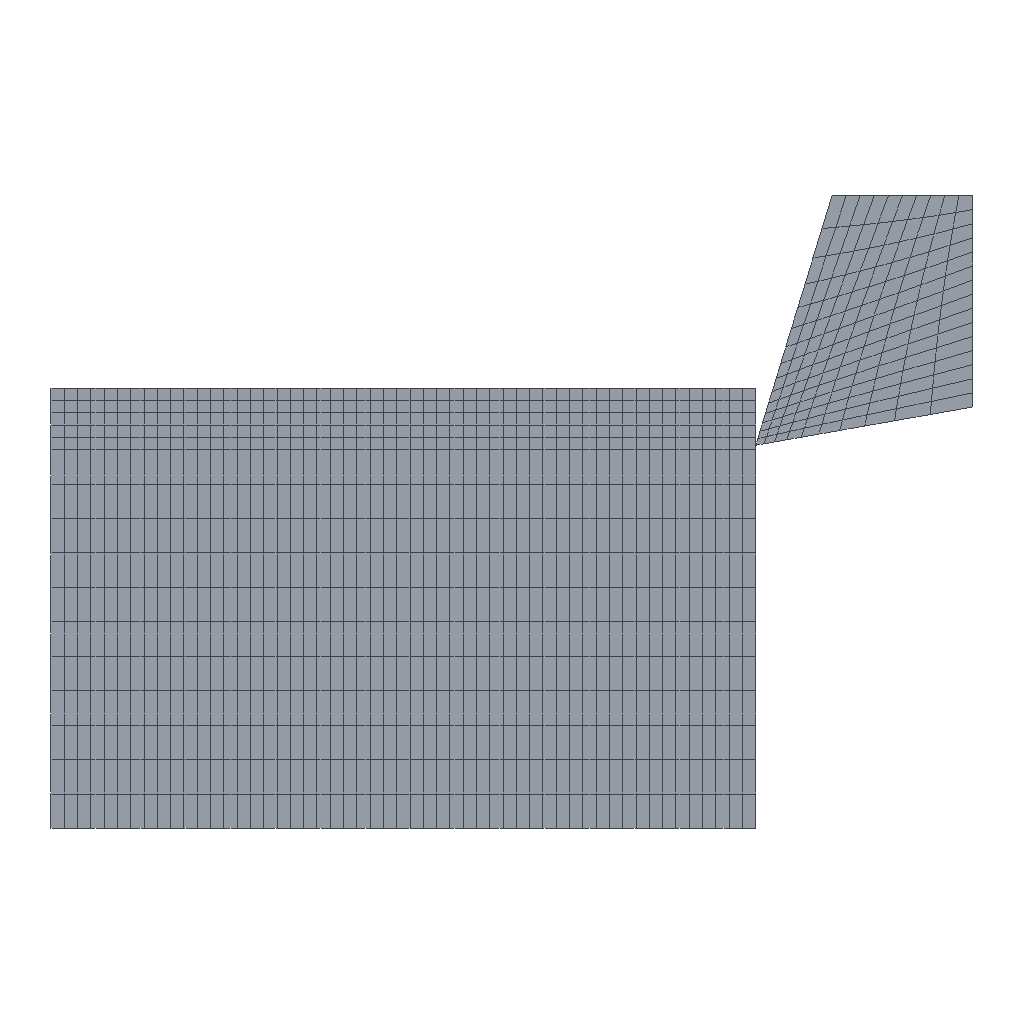Simulation study | abaqus
Set-up summary:
category,name,step,type,value,unit,region
solver,abaqus
solver,version,,,Abaqus/Explicit 2020
units,not stated in the deck,,not stated
analysis,deck,,dynamic temperature-displacement,dynamic temperature-displacement
load_step,Step-1,Step-1,dynamic temperature-displacement
load_step,requested,,,1
mesh,nodes,,,1094
mesh,elements,,,998
element_type,CPE4RT,,plane,998
load,load commands in deck,,count,1
bc,support commands in deck,,count,4
material,CFRP,,in results
material,CFRP-COPY,,in results
material,TOOL,,in results
check,setup vs results,,match,"per instance, exact: element labels, types and connectivity; labels of the nodes the elements use; coordinates of those nodes at SINGLE_PRECISION in 2 of 2 instance(s)"
Abaqus input file, long lists of numbers shortened:
*Heading
** Job name: Job-3 Model name: Model-1-Copy2
** Generated by: Abaqus/CAE 2020
*Preprint, echo=NO, model=NO, history=NO, contact=NO
**
** PARTS
**
*Part, name=tool
*Node
      1,           0.,           0.
      2,  0.9701,  0.1711
** (174 more lines like these left out)
*Element, type=CPE4RT
  1,   1,   2,  13,  12
  2,   2,   3,  14,  13
** (148 more lines like these left out)
*Nset, nset=Set-1, generate
   1,  176,    1
*Elset, elset=Set-1, generate
   1,  150,    1
** Section: tool
*Solid Section, elset=Set-1, material=tool
,
*End Part
**
*Part, name=work
*Node
      1,          80.,          -7.
      2,           0.,          -7.
** (916 more lines like these left out)
*Element, type=CPE4RT
  1,   1,   7, 191, 130
  2,   7,   8, 192, 191
** (846 more lines like these left out)
*Nset, nset=Set-8
   1,   2,   5,   6,   7,   8,   9,  10,  11,  12,  13,  14,  15,  16,  17,  18
  19,  20,  21,  22,  23,  24,  25,  26,  27,  28,  29,  30,  31,  32,  33,  34
** (19 more lines like these left out)
*Elset, elset=Set-8, generate
 584,  848,    1
*Nset, nset=Set-9
   1,   2,   3,   4,   7,   8,   9,  10,  11,  12,  13,  14,  15,  16,  17,  18
  19,  20,  21,  22,  23,  24,  25,  26,  27,  28,  29,  30,  31,  32,  33,  34
** (39 more lines like these left out)
*Elset, elset=Set-9, generate
   1,  583,    1
*Orientation, name=Ori-1
1., 0., 0., 0., 1., 0.
3, 0.
** Section: Section-3
*Solid Section, elset=Set-9, orientation=Ori-1, material=cfrp-Copy
,
** Section: tool
*Solid Section, elset=Set-8, orientation=Ori-1, material=tool
,
*End Part
**
**
** ASSEMBLY
**
*Assembly, name=Assembly
**
*Instance, name=tool-1, part=tool
         80.,         -6.5,           0.
*End Instance
**
*Instance, name=work-1, part=work
*End Instance
**
*Node
      1,   104.667,    21.85,           0.
*Nset, nset=Set-1, instance=work-1
   2,   3,   4,  59,  60,  61,  62,  63,  64,  65,  66,  67,  68,  69,  70,  71
  72,  73,  74,  75,  76,  77,  78,  79,  80,  81,  82,  83,  84,  85,  86,  87
** (3 more lines like these left out)
*Elset, elset=Set-1, instance=work-1
  53, 106, 159, 212, 265, 318, 371, 424, 477, 530, 531, 532, 533, 534, 535, 536
 537, 538, 539, 540, 541, 542, 543, 544, 545, 546, 547, 548, 549, 550, 551, 552
** (2 more lines like these left out)
*Nset, nset=Set-5
 1,
*Nset, nset=Set-6
 1,
*Nset, nset=Set-7, instance=work-1
   3,   4,  69,  70,  71,  72,  73,  74,  75,  76,  77,  78,  79,  80,  81,  82
  83,  84,  85,  86,  87,  88,  89,  90,  91,  92,  93,  94,  95,  96,  97,  98
** (2 more lines like these left out)
*Elset, elset=Set-7, instance=work-1, generate
 531,  583,    1
*Nset, nset=Set-8, instance=work-1
   2,   3,   4,  59,  60,  61,  62,  63,  64,  65,  66,  67,  68,  69,  70,  71
  72,  73,  74,  75,  76,  77,  78,  79,  80,  81,  82,  83,  84,  85,  86,  87
** (3 more lines like these left out)
*Elset, elset=Set-8, instance=work-1
  53, 106, 159, 212, 265, 318, 371, 424, 477, 530, 531, 532, 533, 534, 535, 536
 537, 538, 539, 540, 541, 542, 543, 544, 545, 546, 547, 548, 549, 550, 551, 552
** (2 more lines like these left out)
*Nset, nset=b_Set-2, instance=tool-1, generate
   1,  176,    1
*Elset, elset=b_Set-2, instance=tool-1, generate
   1,  150,    1
*Nset, nset=s_Set-4, instance=work-1
   1,   2,   3,   4,   5,   6,   7,   8,   9,  10,  11,  12,  13,  14,  15,  16
  17,  18,  19,  20,  21,  22,  23,  24,  25,  26,  27,  28,  29,  30,  31,  32
** (42 more lines like these left out)
*Elset, elset=s_Set-4, instance=work-1
   1,   2,   3,   4,   5,   6,   7,   8,   9,  10,  11,  12,  13,  14,  15,  16
  17,  18,  19,  20,  21,  22,  23,  24,  25,  26,  27,  28,  29,  30,  31,  32
** (38 more lines like these left out)
*Nset, nset=_PickedSet9, internal
 1,
*Elset, elset=_m_Surf-1_S1, internal, instance=tool-1, generate
  1,  10,   1
*Elset, elset=_m_Surf-1_S4, internal, instance=tool-1, generate
   1,  141,   10
*Surface, type=ELEMENT, name=m_Surf-1
_m_Surf-1_S1, S1
_m_Surf-1_S4, S4
** Constraint: Constraint-1
*Rigid Body, ref node=_PickedSet9, elset=b_Set-2
*End Assembly
*Amplitude, name=Amp-1
             0.,              0.,              1.,              1.
**
** MATERIALS
**
*Material, name=cfrp
*Conductivity
 0.5,
*Damage Initiation, criterion=HASHIN
518.,257., 29., 76., 37., 27.
*Damage Evolution, type=ENERGY
20.,20.,20.,20.
*Density
 2e-09,
*Elastic, type=ENGINEERING CONSTANTS
54000.,54000.,54000.,  0.25,  0.35,  0.35,16000.,24000.
24000.,
*Specific Heat
 8e+08,
*Material, name=cfrp-Copy
*Conductivity
 0.5,
*Density
 2e-09,
*Elastic, type=ENGINEERING CONSTANTS
54000.,54000.,54000.,  0.25,  0.35,  0.35,16000.,24000.
24000.,
*Specific Heat
 8e+08,
*Material, name=tool
*Conductivity
45.,
*Density
 7.8e-09,
*Elastic
210000., 0.3
*Specific Heat
 4.6e+08,
**
** INTERACTION PROPERTIES
**
*Surface Interaction, name=IntProp-1
*Friction
 0.2,
*Surface Behavior, pressure-overclosure=HARD
*Gap Conductance
 0.1,    0.
  0., 0.001
** ----------------------------------------------------------------
**
** STEP: Step-1
**
*Step, name=Step-1, nlgeom=YES
*Dynamic Temperature-displacement, Explicit
, 1.
*Bulk Viscosity
0.06, 1.2
** Mass Scaling: Semi-Automatic
**               Whole Model
*Fixed Mass Scaling, factor=50.
**
** BOUNDARY CONDITIONS
**
** Name: BC-1 Type: 对称/反对称/完全固定
*Boundary
Set-8, ENCASTRE
** Name: [REDACTED] : Displacement/rotation angle
*Boundary, amplitude=Amp-1
Set-6, 1, 1, -80.
Set-6, 2, 2
Set-6, 6, 6
**
** INTERACTIONS
**
** Interaction: Int-2
*Contact, op=NEW
*Contact Inclusions, ALL EXTERIOR
*Contact Property Assignment
 ,  , IntProp-1
**
** OUTPUT REQUESTS
**
*Restart, write, number interval=1, time marks=NO
**
** FIELD OUTPUT: F-Output-1
**
*Output, field, number interval=50
*Node Output
CF, NT, RF, RM, RT, U, V
*Element Output, directions=YES
DAMAGEC, DAMAGET, E, LE, MISES, MISESMAX, MISESONLY, PE, PEEQ, PEEQMAX, PEEQT, PRESSONLY, S, SDEG, SEQUT, SF
SSAVG, STATUS, SVAVG, TEMP, YIELDPOT
*Contact Output
CDISP, CSTRESS
**
** HISTORY OUTPUT: H-Output-1
**
*Output, history, frequency=1
*Node Output, nset=Set-5
RF1, RF2
*End Step
Results summary:
result,step,Step-1,partial,increments=159782 time=0.2096/1.0
result,analysis,,,"dynamic temperature-displacement, explict"
result,last_loadstep,,,1
result,primary field,,,"U, NT11"
result,reaction total,,FX,-164472.803,model units
result,reaction total,,FY,-24677.193,model units
result,reaction total,,FZ,0.0,model units